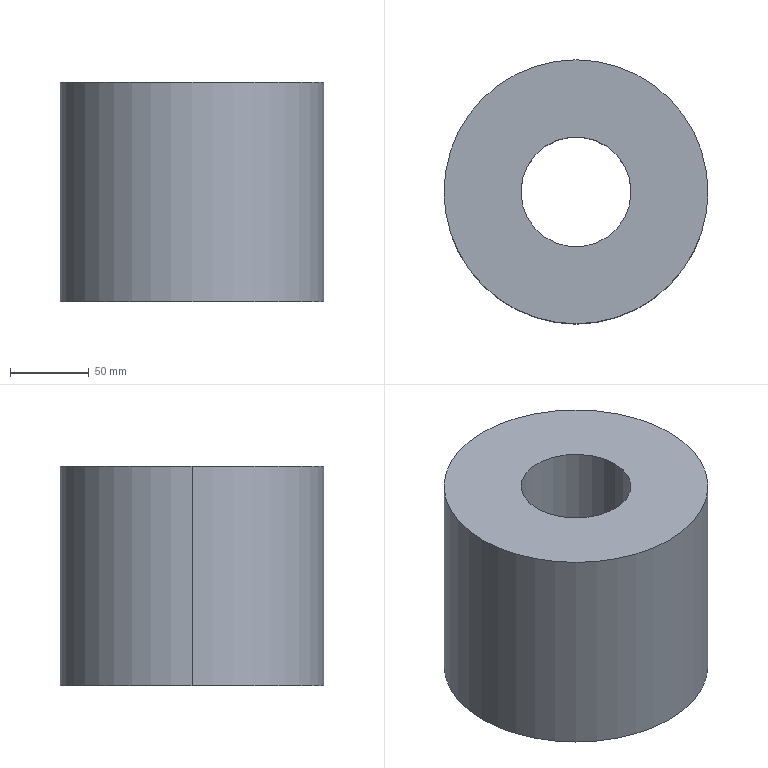Part | SolidWorks | features Extrusion 1 | 1 solid | 6 faces | box 168 x 168 x 140 mm | volume 2564608 mm3 | cylinder 4 | plane 2 | commonest cylinder face diameters 70 x2 168 x2
STEP:
#1=CARTESIAN_POINT('',(-35.,0.,70.));
#2=VERTEX_POINT('',#1);
#3=CARTESIAN_POINT('',(35.,0.,70.));
#4=VERTEX_POINT('',#3);
#5=CARTESIAN_POINT('',(0.,0.,70.));
#6=DIRECTION('',(0.,0.,1.));
#7=DIRECTION('',(1.,0.,0.));
#8=AXIS2_PLACEMENT_3D('',#5,#6,#7);
#9=CIRCLE('',#8,35.);
#10=EDGE_CURVE('',#2,#4,#9,.T.);
#11=ORIENTED_EDGE('',*,*,#10,.T.);
#12=CARTESIAN_POINT('',(35.,0.,-70.));
#13=VERTEX_POINT('',#12);
#14=CARTESIAN_POINT('',(35.,0.,70.));
#15=DIRECTION('',(0.,0.,-1.));
#16=VECTOR('',#15,1000.);
#17=LINE('',#14,#16);
#18=EDGE_CURVE('',#4,#13,#17,.T.);
#19=ORIENTED_EDGE('',*,*,#18,.T.);
#20=CARTESIAN_POINT('',(-35.,0.,-70.));
#21=VERTEX_POINT('',#20);
#22=CARTESIAN_POINT('',(0.,0.,-70.));
#23=DIRECTION('',(0.,0.,1.));
#24=DIRECTION('',(1.,0.,0.));
#25=AXIS2_PLACEMENT_3D('',#22,#23,#24);
#26=CIRCLE('',#25,35.);
#27=EDGE_CURVE('',#21,#13,#26,.T.);
#28=ORIENTED_EDGE('',*,*,#27,.F.);
#29=CARTESIAN_POINT('',(-35.,0.,70.));
#30=DIRECTION('',(0.,0.,-1.));
#31=VECTOR('',#30,1000.);
#32=LINE('',#29,#31);
#33=EDGE_CURVE('',#2,#21,#32,.T.);
#34=ORIENTED_EDGE('',*,*,#33,.F.);
#35=EDGE_LOOP('',(#11,#19,#28,#34));
#36=FACE_OUTER_BOUND('',#35,.T.);
#37=CARTESIAN_POINT('',(0.,0.,70.));
#38=DIRECTION('',(0.,0.,-1.));
#39=DIRECTION('',(-1.,0.,0.));
#40=AXIS2_PLACEMENT_3D('',#37,#38,#39);
#41=CYLINDRICAL_SURFACE('',#40,35.);
#42=ADVANCED_FACE('',(#36),#41,.F.);
#43=CARTESIAN_POINT('',(84.,0.,70.));
#44=VERTEX_POINT('',#43);
#45=CARTESIAN_POINT('',(-84.,0.,70.));
#46=VERTEX_POINT('',#45);
#47=CARTESIAN_POINT('',(0.,0.,70.));
#48=DIRECTION('',(0.,0.,1.));
#49=DIRECTION('',(1.,0.,0.));
#50=AXIS2_PLACEMENT_3D('',#47,#48,#49);
#51=CIRCLE('',#50,84.);
#52=EDGE_CURVE('',#44,#46,#51,.T.);
#53=ORIENTED_EDGE('',*,*,#52,.F.);
#54=CARTESIAN_POINT('',(84.,0.,-70.));
#55=VERTEX_POINT('',#54);
#56=CARTESIAN_POINT('',(84.,0.,70.));
#57=DIRECTION('',(0.,0.,-1.));
#58=VECTOR('',#57,1000.);
#59=LINE('',#56,#58);
#60=EDGE_CURVE('',#44,#55,#59,.T.);
#61=ORIENTED_EDGE('',*,*,#60,.T.);
#62=CARTESIAN_POINT('',(-84.,0.,-70.));
#63=VERTEX_POINT('',#62);
#64=CARTESIAN_POINT('',(0.,0.,-70.));
#65=DIRECTION('',(0.,0.,1.));
#66=DIRECTION('',(1.,0.,0.));
#67=AXIS2_PLACEMENT_3D('',#64,#65,#66);
#68=CIRCLE('',#67,84.);
#69=EDGE_CURVE('',#55,#63,#68,.T.);
#70=ORIENTED_EDGE('',*,*,#69,.T.);
#71=CARTESIAN_POINT('',(-84.,0.,70.));
#72=DIRECTION('',(0.,0.,-1.));
#73=VECTOR('',#72,1000.);
#74=LINE('',#71,#73);
#75=EDGE_CURVE('',#46,#63,#74,.T.);
#76=ORIENTED_EDGE('',*,*,#75,.F.);
#77=EDGE_LOOP('',(#53,#61,#70,#76));
#78=FACE_OUTER_BOUND('',#77,.T.);
#79=CARTESIAN_POINT('',(0.,0.,70.));
#80=DIRECTION('',(0.,0.,-1.));
#81=DIRECTION('',(-1.,0.,0.));
#82=AXIS2_PLACEMENT_3D('',#79,#80,#81);
#83=CYLINDRICAL_SURFACE('',#82,84.);
#84=ADVANCED_FACE('',(#78),#83,.T.);
#85=CARTESIAN_POINT('',(0.,0.,70.));
#86=DIRECTION('',(0.,0.,1.));
#87=DIRECTION('',(1.,0.,0.));
#88=AXIS2_PLACEMENT_3D('',#85,#86,#87);
#89=CIRCLE('',#88,84.);
#90=EDGE_CURVE('',#46,#44,#89,.T.);
#91=ORIENTED_EDGE('',*,*,#90,.T.);
#92=ORIENTED_EDGE('',*,*,#52,.T.);
#93=EDGE_LOOP('',(#91,#92));
#94=FACE_OUTER_BOUND('',#93,.T.);
#95=ORIENTED_EDGE('',*,*,#10,.F.);
#96=CARTESIAN_POINT('',(0.,0.,70.));
#97=DIRECTION('',(0.,0.,1.));
#98=DIRECTION('',(1.,0.,0.));
#99=AXIS2_PLACEMENT_3D('',#96,#97,#98);
#100=CIRCLE('',#99,35.);
#101=EDGE_CURVE('',#4,#2,#100,.T.);
#102=ORIENTED_EDGE('',*,*,#101,.F.);
#103=EDGE_LOOP('',(#95,#102));
#104=FACE_BOUND('',#103,.T.);
#105=CARTESIAN_POINT('',(0.,0.,70.));
#106=DIRECTION('',(0.,0.,1.));
#107=DIRECTION('',(1.,0.,0.));
#108=AXIS2_PLACEMENT_3D('',#105,#106,#107);
#109=PLANE('',#108);
#110=ADVANCED_FACE('',(#94,#104),#109,.T.);
#111=CARTESIAN_POINT('',(0.,0.,-70.));
#112=DIRECTION('',(0.,0.,1.));
#113=DIRECTION('',(1.,0.,0.));
#114=AXIS2_PLACEMENT_3D('',#111,#112,#113);
#115=CIRCLE('',#114,84.);
#116=EDGE_CURVE('',#63,#55,#115,.T.);
#117=ORIENTED_EDGE('',*,*,#116,.F.);
#118=ORIENTED_EDGE('',*,*,#69,.F.);
#119=EDGE_LOOP('',(#117,#118));
#120=FACE_OUTER_BOUND('',#119,.T.);
#121=ORIENTED_EDGE('',*,*,#27,.T.);
#122=CARTESIAN_POINT('',(0.,0.,-70.));
#123=DIRECTION('',(0.,0.,1.));
#124=DIRECTION('',(1.,0.,0.));
#125=AXIS2_PLACEMENT_3D('',#122,#123,#124);
#126=CIRCLE('',#125,35.);
#127=EDGE_CURVE('',#13,#21,#126,.T.);
#128=ORIENTED_EDGE('',*,*,#127,.T.);
#129=EDGE_LOOP('',(#121,#128));
#130=FACE_BOUND('',#129,.T.);
#131=CARTESIAN_POINT('',(0.,0.,-70.));
#132=DIRECTION('',(0.,0.,1.));
#133=DIRECTION('',(1.,0.,0.));
#134=AXIS2_PLACEMENT_3D('',#131,#132,#133);
#135=PLANE('',#134);
#136=ADVANCED_FACE('',(#120,#130),#135,.F.);
#137=ORIENTED_EDGE('',*,*,#60,.F.);
#138=ORIENTED_EDGE('',*,*,#90,.F.);
#139=ORIENTED_EDGE('',*,*,#75,.T.);
#140=ORIENTED_EDGE('',*,*,#116,.T.);
#141=EDGE_LOOP('',(#137,#138,#139,#140));
#142=FACE_OUTER_BOUND('',#141,.T.);
#143=CARTESIAN_POINT('',(0.,0.,70.));
#144=DIRECTION('',(0.,0.,-1.));
#145=DIRECTION('',(-1.,0.,0.));
#146=AXIS2_PLACEMENT_3D('',#143,#144,#145);
#147=CYLINDRICAL_SURFACE('',#146,84.);
#148=ADVANCED_FACE('',(#142),#147,.T.);
#149=ORIENTED_EDGE('',*,*,#18,.F.);
#150=ORIENTED_EDGE('',*,*,#101,.T.);
#151=ORIENTED_EDGE('',*,*,#33,.T.);
#152=ORIENTED_EDGE('',*,*,#127,.F.);
#153=EDGE_LOOP('',(#149,#150,#151,#152));
#154=FACE_OUTER_BOUND('',#153,.T.);
#155=CARTESIAN_POINT('',(0.,0.,70.));
#156=DIRECTION('',(0.,0.,-1.));
#157=DIRECTION('',(-1.,0.,0.));
#158=AXIS2_PLACEMENT_3D('',#155,#156,#157);
#159=CYLINDRICAL_SURFACE('',#158,35.);
#160=ADVANCED_FACE('',(#154),#159,.F.);
#161=CLOSED_SHELL('',(#42,#84,#110,#136,#148,#160));
#162=MANIFOLD_SOLID_BREP('',#161);
#163=CARTESIAN_POINT('',(0.,0.,0.));
#164=DIRECTION('',(0.,0.,1.));
#165=DIRECTION('',(1.,0.,0.));
#166=AXIS2_PLACEMENT_3D('',#163,#164,#165);
#167=(LENGTH_UNIT()NAMED_UNIT(*)SI_UNIT(.MILLI.,.METRE.));
#168=UNCERTAINTY_MEASURE_WITH_UNIT(LENGTH_MEASURE(0.00001),#167,'','');
#169=(NAMED_UNIT(*)PLANE_ANGLE_UNIT()SI_UNIT($,.RADIAN.));
#170=(NAMED_UNIT(*)SI_UNIT($,.STERADIAN.)SOLID_ANGLE_UNIT());
#171=(GEOMETRIC_REPRESENTATION_CONTEXT(3)GLOBAL_UNCERTAINTY_ASSIGNED_CONTEXT((#168))GLOBAL_UNIT_ASSIGNED_CONTEXT((#167,#169,#170))REPRESENTATION_CONTEXT('',''));
#172=ADVANCED_BREP_SHAPE_REPRESENTATION('',(#162,#166),#171);